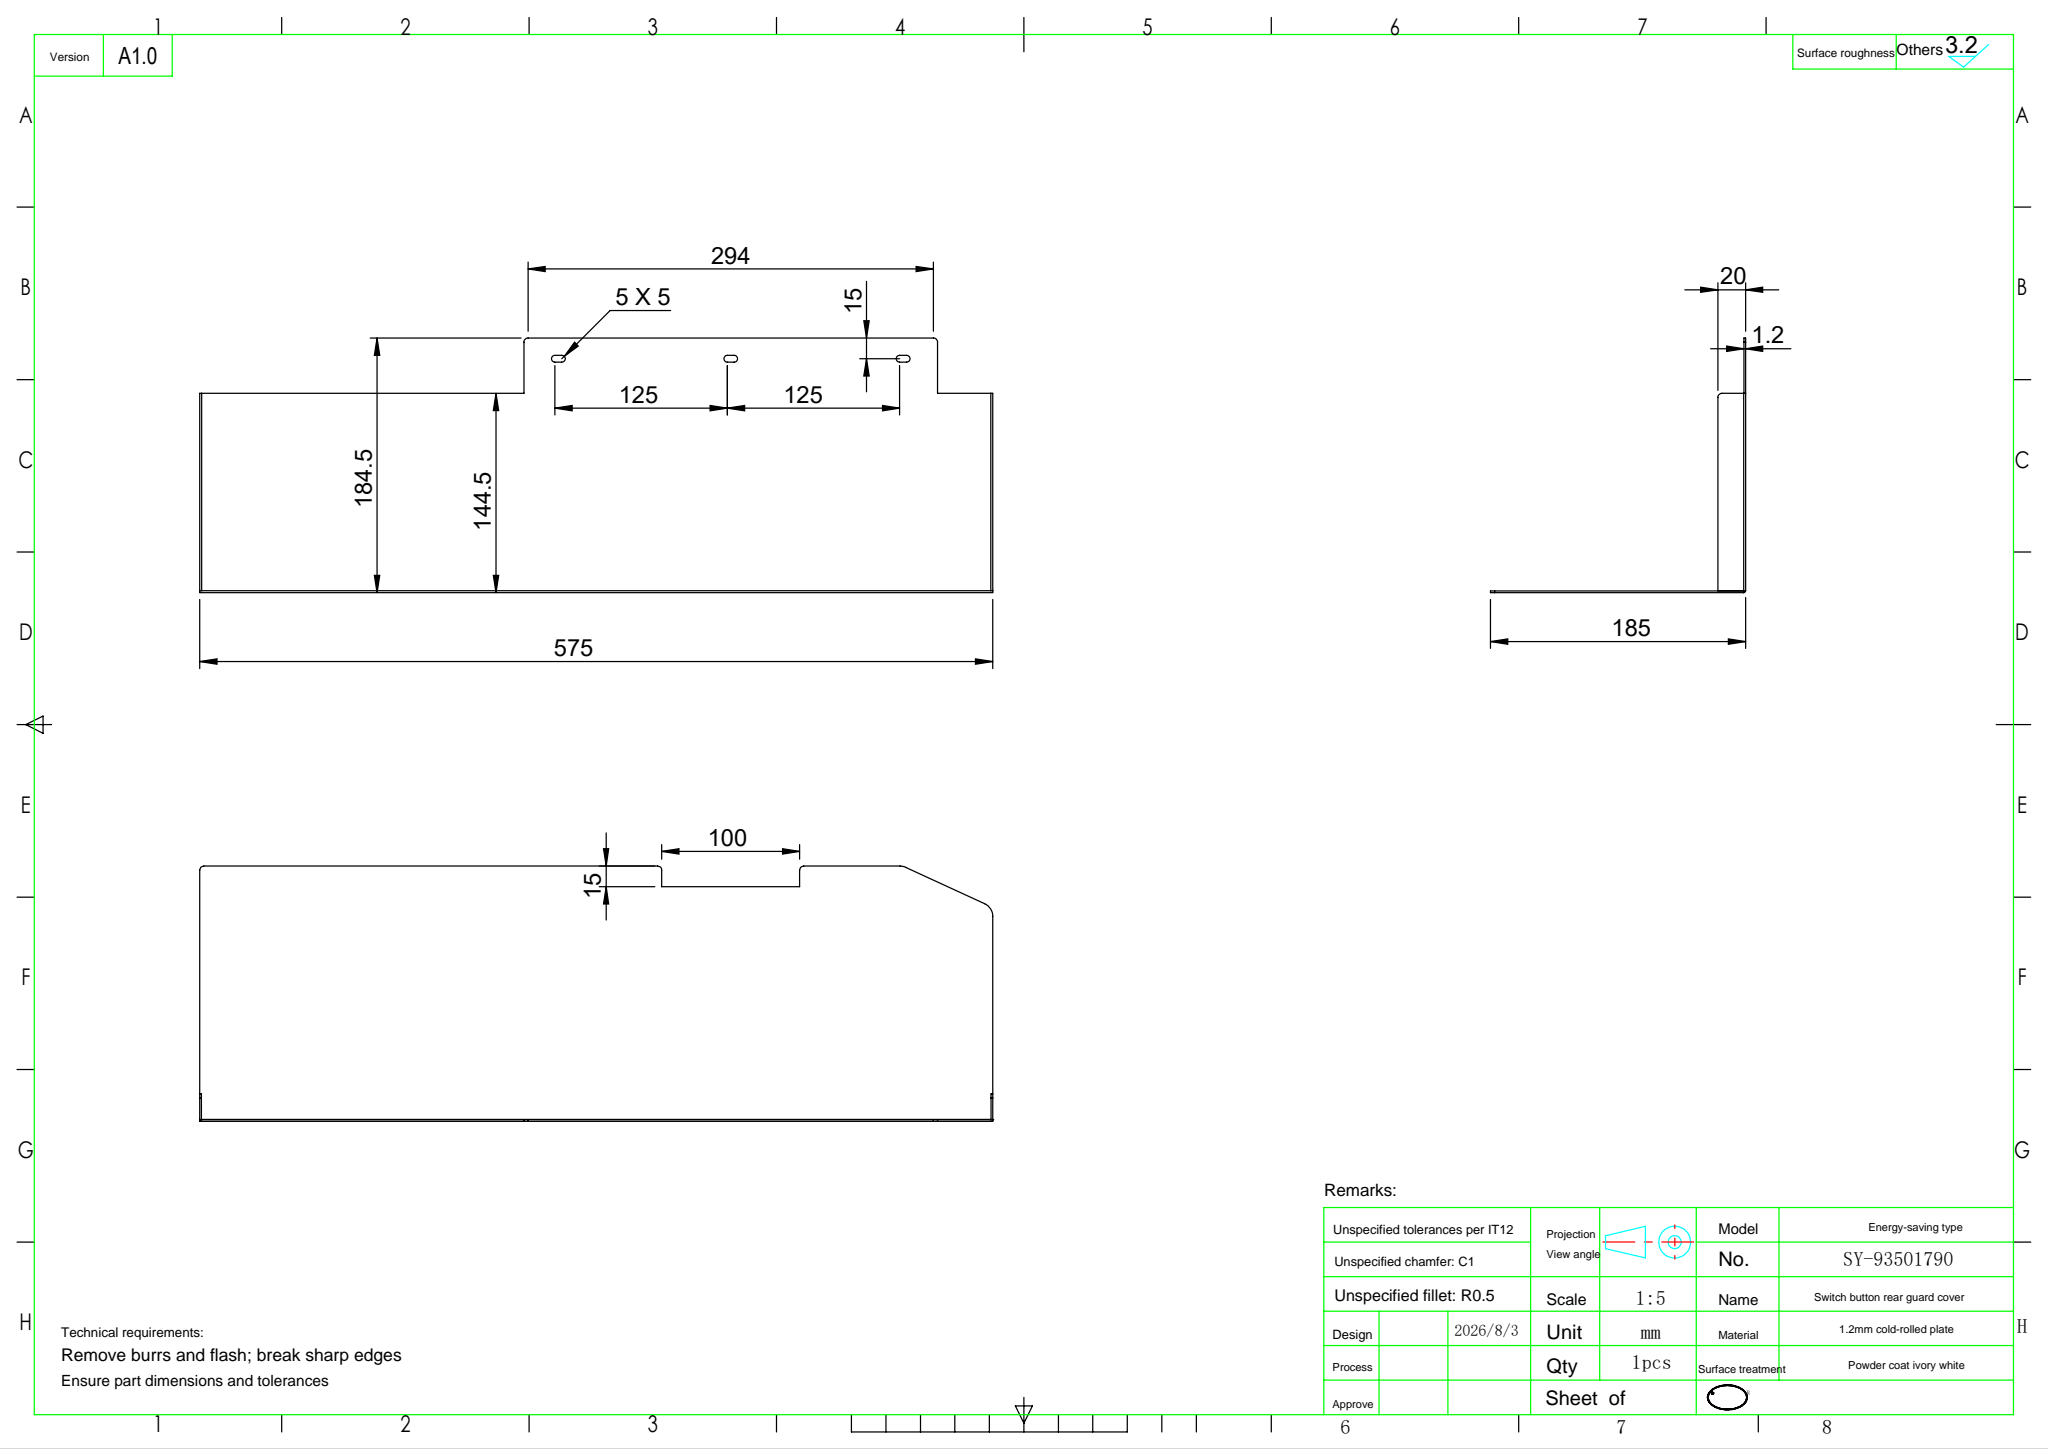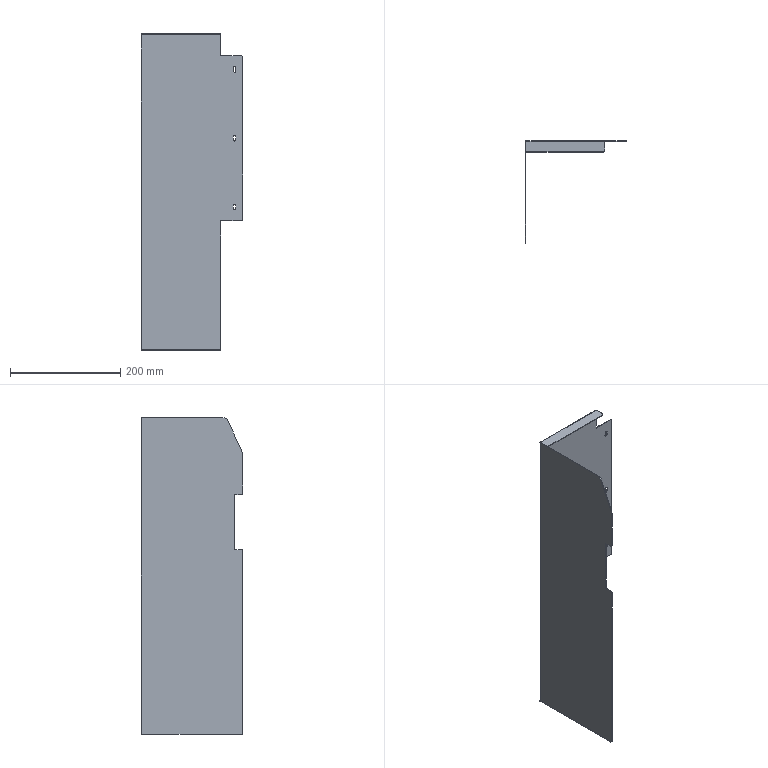Part | SolidWorks | features ICE 4, Fillet 2, EdgeFlange 1, FlatPattern 1, LPattern 1, MoveFace 1, SMBaseFlange 1, SheetMetal 1 | 1 solid | 58 faces | box 184.5 x 185 x 575 mm | volume 243873 mm3 | plane 37 | cylinder 21 | commonest cylinder face diameters 6 x7 5 x6 0.4 x3 2.8 x3 20 x2